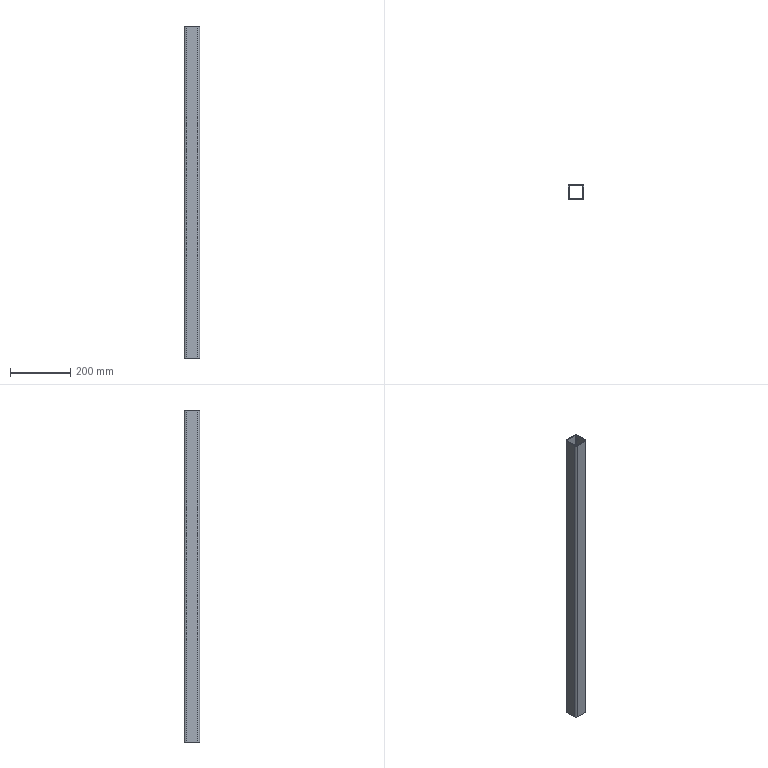Part | SolidWorks | features HoleWzd 4, WeldMemberFeat 1, WeldmentFeature 1 | 1 solid | 54 faces | box 50 x 50 x 1100 mm | volume 594018 mm3 | cylinder 44 | plane 10 | commonest cylinder face diameters 4.2 x20 5 x16 6 x4 12 x4